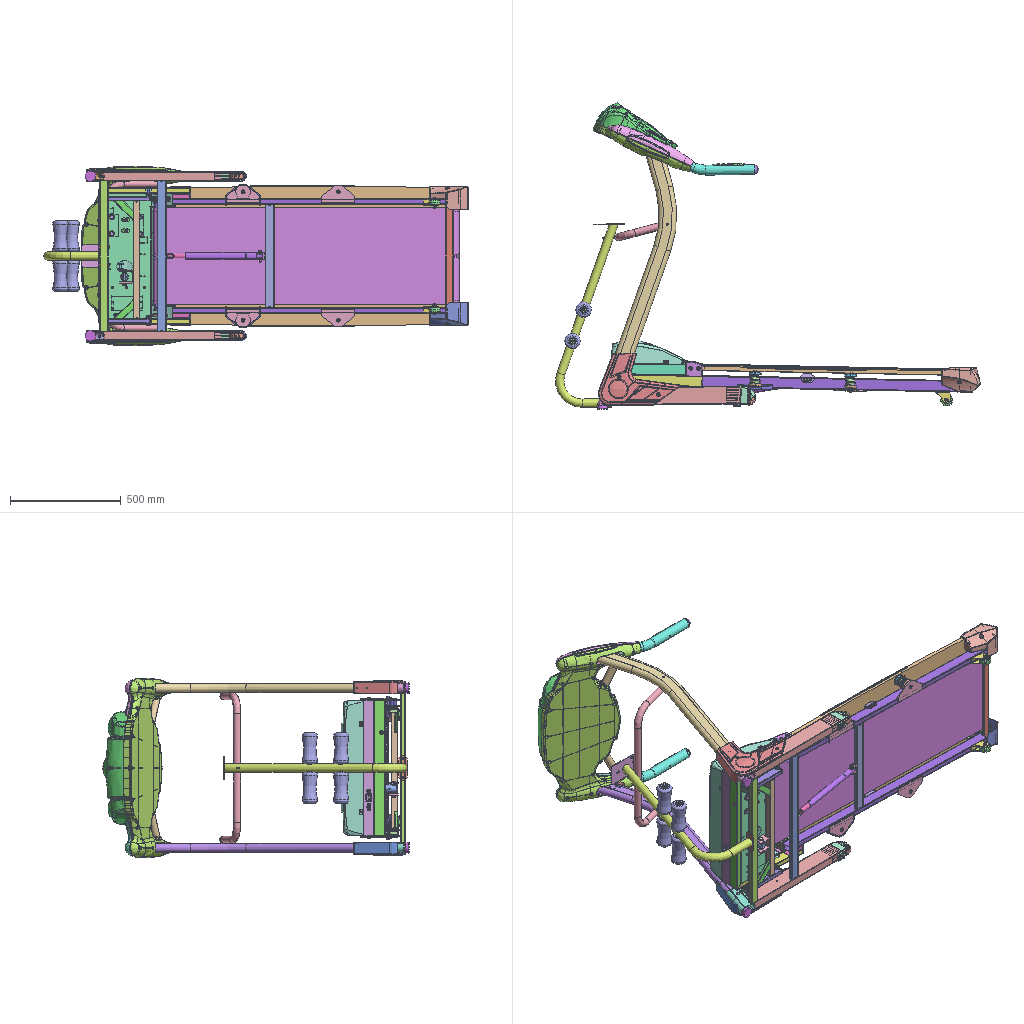Assembly | STEP file | 145 different items | 312 placed | box 1916 x 1381 x 810 mm
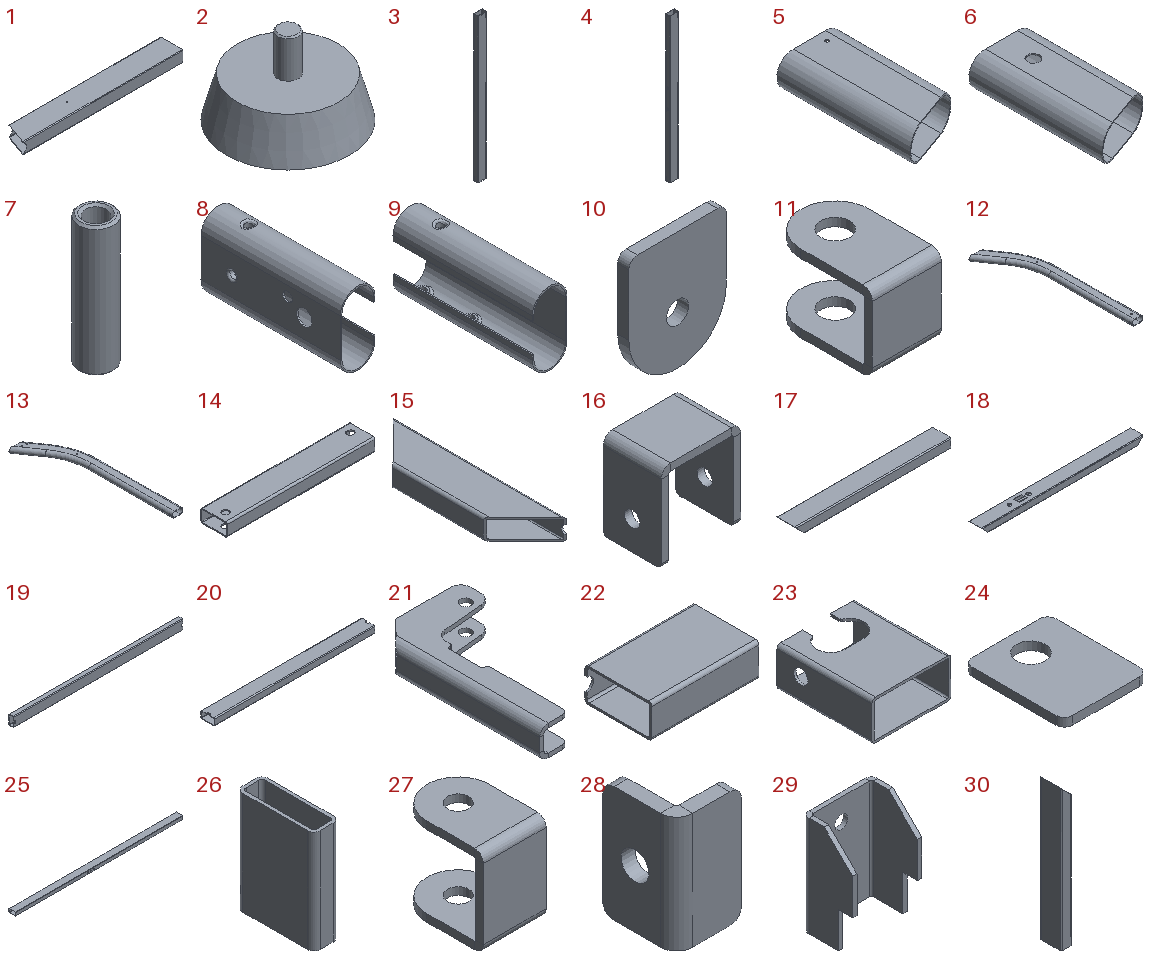Parts list (item | name | quantity | parent item | size | volume):
1 | 6150101 | x2 | in 6150100 | 569.929 x 80 x 40 mm | 191514 mm3
2 | 6150101W | x2 | in 6150100Z | 48.593 x 48.593 x 32 mm | 27204 mm3
3 | 6150102 | x1 | in 6150100 | 40 x 20 x 680 mm | 113098 mm3
4 | 6150103 | x1 | in 6150100 | 40 x 20 x 680 mm | 112626 mm3
5 | 6150104L | x1 | in 6150100 | 80 x 165 x 40 mm | 45327 mm3
6 | 6150104R | x1 | in 6150100 | 80 x 165 x 40 mm | 45081 mm3
7 | 6150104W | x2 | in 6150102LWZ, 6150102RWZ | 8.2 x 8.2 x 31 mm | 968.239 mm3
8 | 6150105L | x1 | in 6150100 | 36 x 145 x 76 mm | 34893 mm3
9 | 6150105R | x1 | in 6150100 | 36 x 145 x 76 mm | 34904 mm3
10 | 6150107 | x2 | in 6150100 | 35 x 4 x 42.5 mm | 5208 mm3
11 | 6150108 | x4 | in 6150100, 6150500 | 25 x 38.5 x 28 mm | 6374 mm3
12 | 6150201L | x1 | in 615 | 263.127 x 990.805 x 40 mm | 310034 mm3
13 | 6150201R | x1 | in 615 | 263.127 x 990.805 x 40 mm | 310034 mm3
14 | 6150402 | x2 | in 6150400 | 225 x 40 x 20 mm | 36971 mm3
15 | 6150403 | x2 | in 6150400 | 30 x 125 x 15 mm | 9413 mm3
16 | 6150404 | x1 | in 6150400 | 55 x 40 x 60 mm | 31409 mm3
17 | 6150501 | x2 | in 6150500 | 410 x 50 x 25 mm | 84495 mm3
18 | 6150502 | x1 | in 6150500 | 613 x 50 x 25 mm | 116984 mm3
19 | 6150504 | x1 | in 6150500 | 515 x 15 x 30 mm | 62451 mm3
20 | 6150505 | x1 | in 6150500 | 465 x 40 x 20 mm | 77302 mm3
21 | 6150506 | x1 | in 6150500 | 84 x 160 x 29 mm | 53248 mm3
22 | 6150507 | x2 | in 6150500 | 80 x 50 x 25 mm | 16946 mm3
23 | 6150508 | x1 | in 6150500 | 50 x 60 x 25 mm | 11554 mm3
24 | 6150509 | x1 | in 6150500 | 50 x 60 x 5 mm | 13731 mm3
25 | 6150510 | x2 | in 6150500 | 1235 x 50 x 25 mm | 262357 mm3
26 | 6150511 | x2 | in 6150500 | 10 x 30 x 40 mm | 3453 mm3
27 | 6150512 | x1 | in 6150500 | 25 x 35 x 35 mm | 6553 mm3
28 | 6150513 | x4 | in 6150500 | 14 x 16 x 25 mm | 1860 mm3
29 | 6150514 | x4 | in 6150500 | 48 x 35 x 70 mm | 19897 mm3
30 | 6150515 | x1 | in 6150500 | 25 x 50 x 334 mm | 67995 mm3
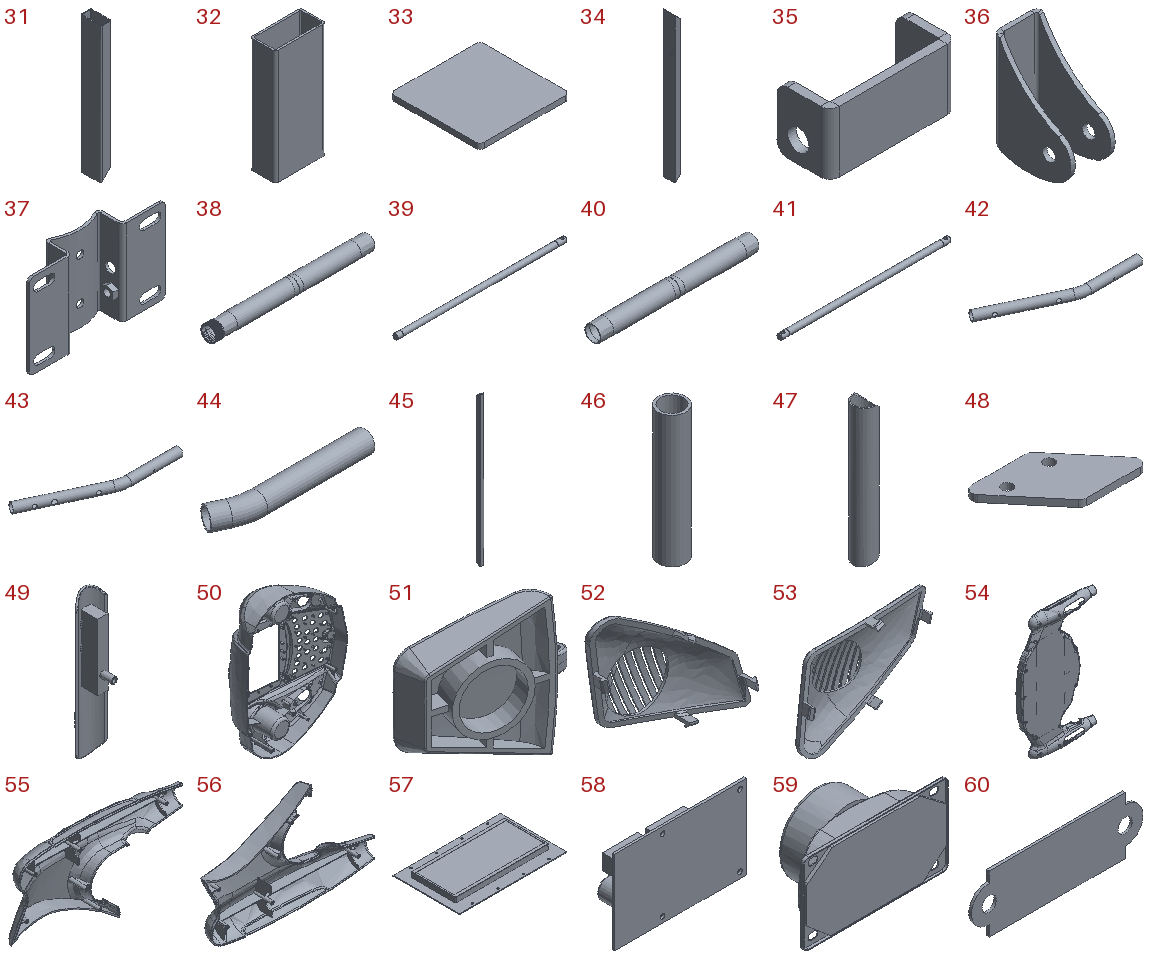31 | 6150516 | x1 | in 6150500 | 25 x 50 x 334 mm | 67613 mm3
32 | 6150517 | x2 | in 6150500 | 40 x 20 x 90 mm | 14984 mm3
33 | 6150518 | x2 | in 6150500 | 50 x 50 x 3 mm | 7484 mm3
34 | 6150519 | x1 | in 6150500 | 25 x 50 x 613 mm | 123960 mm3
35 | 6150521 | x2 | in 6150500 | 60 x 25 x 29 mm | 10869 mm3
36 | 6150522 | x2 | in 6150500 | 30 x 53 x 70.522 mm | 17329 mm3
37 | 6150601 | x1 | in 6150600Z | 160 x 30 x 100 mm | 59957 mm3
38 | 6150701 | x1 | in 6150700Z | 515 x 50 x 50 mm | 250147 mm3
39 | 6150702 | x1 | in 6150700Z | 565 x 17 x 17 mm | 128550 mm3
40 | 6150801 | x1 | in 6150800Z | 475 x 50 x 50 mm | 235448 mm3
41 | 6150802 | x1 | in 6150800Z | 523 x 17 x 17 mm | 116773 mm3
42 | 6151201L | x1 | in 6151200 | 584.322 x 188.458 x 38.1 mm | 101738 mm3
43 | 6151201R | x1 | in 6151200 | 584.322 x 188.458 x 38.1 mm | 101253 mm3
44 | 6151201WA | x2 | in 6151200Z | 313.697 x 67.391 x 44.1 mm | 119753 mm3
45 | 6151202 | x1 | in 6151200 | 20 x 20 x 700 mm | 73457 mm3
46 | 6151202W | x2 | in 6151200Z | 34.6 x 34.6 x 165 mm | 49141 mm3
47 | 6151203 | x2 | in 6151200 | 28.6 x 28.6 x 183 mm | 22465 mm3
48 | 6151204 | x2 | in 6151200 | 82.726 x 50 x 5 mm | 12291 mm3
49 | 6151204W | x2 | in 6151200Z | 31 x 32.516 x 144.3 mm | 20924 mm3
50 | 6151206W | x1 | in 6151200A | 380 x 123.405 x 510 mm | 795942 mm3
51 | 6151207W | x1 | in 6151200A | 35.148 x 15.37 x 38.312 mm | 3411 mm3
52 | 6151208LW | x1 | in 6151200A | 94.278 x 29.99 x 86.4 mm | 11134 mm3
53 | 6151208RW | x1 | in 6151200A | 94.278 x 29.99 x 86.4 mm | 11135 mm3
54 | 6151209W | x1 | in 6151200A | - | -
55 | 6151210LW | x1 | in 6151200A | 418.826 x 58.845 x 246.762 mm | 255227 mm3
56 | 6151210RW | x1 | in 6151200A | 418.823 x 58.845 x 246.762 mm | 256127 mm3
57 | 6151211W | x1 | in 6151200A | 210 x 130 x 11.5 mm | 192424 mm3
58 | 6151212W | x1 | in 6151200A | 85 x 25.5 x 54 mm | 22602 mm3
59 | 6151213W | x2 | in 6151200A | 90 x 37.5 x 50 mm | 46130 mm3
60 | 6151214W | x1 | in 6151200A | 48 x 0.7 x 16 mm | 462.985 mm3
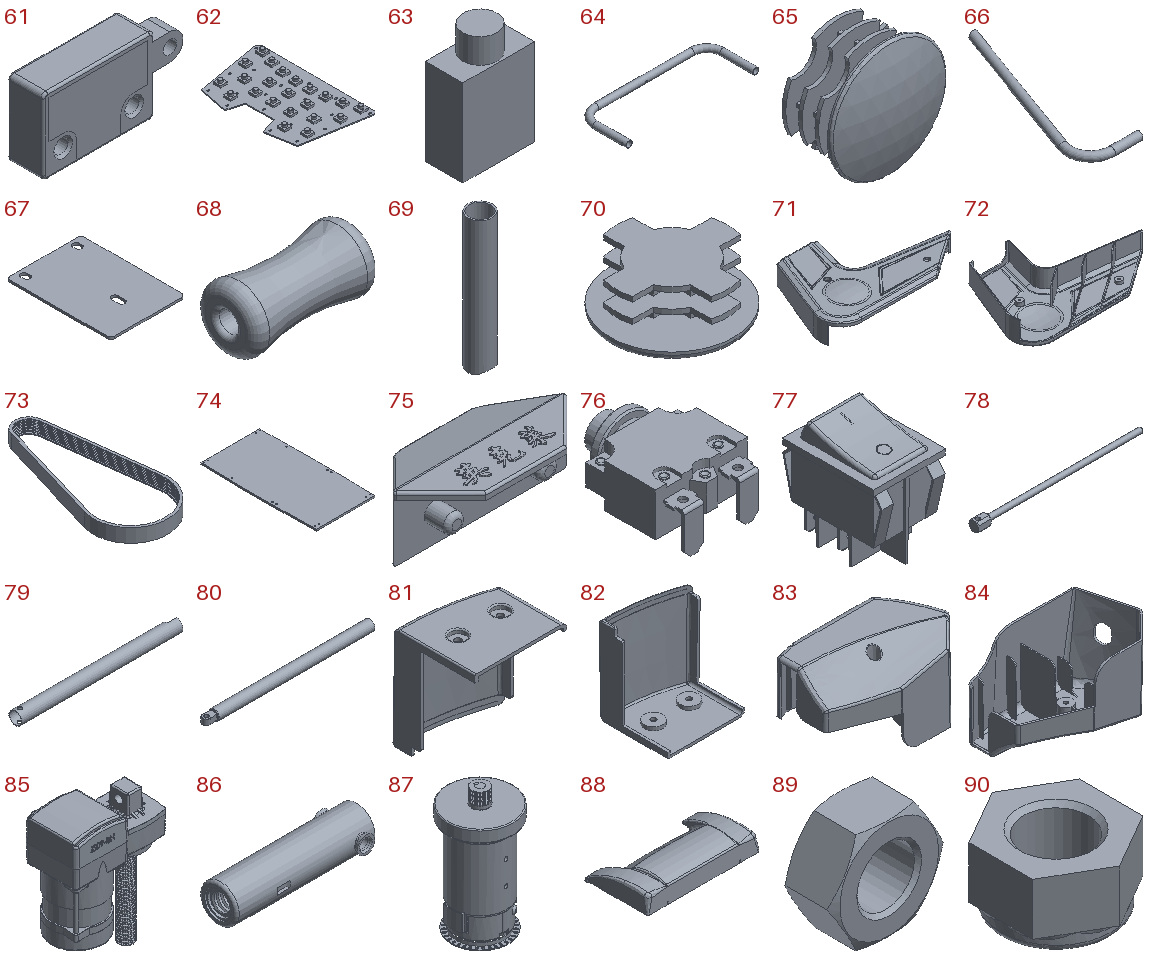61 | 6151215W | x1 | in 6151200A | 31.5 x 8 x 17 mm | 3233 mm3
62 | 6151216W | x1 | in 6151200A | 123.89 x 199.336 x 9.1 mm | 46747 mm3
63 | 6151217W | x1 | in 6151200A | 11.5 x 6 x 18 mm | 1061 mm3
64 | 6151301 | x1 | in 6151300 | 679.8 x 265.9 x 31.8 mm | 153699 mm3
65 | 6151301W | x2 | in 6151300Z | 31.8 x 17.071 x 31.8 mm | 4059 mm3
66 | 6151401 | x1 | in 6151400 | 289.236 x 823.315 x 38.1 mm | 178322 mm3
67 | 6151403 | x1 | in 6151400 | 100 x 140 x 3 mm | 40958 mm3
68 | 6151403W | x4 | in 6151400Z | 140 x 70 x 70 mm | 348651 mm3
69 | 6151404 | x4 | in 6151400 | 25.4 x 25.4 x 140 mm | 15577 mm3
70 | 6151404W | x4 | in 6151400Z | 25.4 x 25.4 x 10 mm | 1636 mm3
71 | BLZHT2-L | x1 | in 615 | 369.553 x 235 x 62.57 mm | 247384 mm3
72 | BLZHT2-R | x1 | in 615 | 369.553 x 235 x 62.57 mm | 247382 mm3
73 | DE200J618 | x1 | in 6150500Z | 99 x 216 x 18 mm | 21820 mm3
74 | DECAK 615 | x1 | in 6150500Z | 633 x 1220 x 18 mm | 13739057 mm3
75 | DECH07 | x2 | in 6150500Z | 74.172 x 40 x 28.5 mm | 30644 mm3
76 | EC002 | x1 | in 6150500Z | 29.3 x 39.3 x 19.65 mm | 10331 mm3
77 | EP002 | x1 | in 6150500Z | 25 x 34.5 x 34.784 mm | 14567 mm3
78 | GAS SHOCK 608S | x1 | in 615 | 353.5 x 20 x 20 mm | 34694 mm3
79 | GAS SHOCK 608W | x1 | in 615 | 353 x 28 x 28 mm | 42661 mm3
80 | GAS SHOCK 608X | x1 | in 615 | 359 x 22 x 22 mm | 94119 mm3
81 | HGL | x1 | in 6150500Z | 76.869 x 67.947 x 85 mm | 33917 mm3
82 | HGR | x1 | in 6150500Z | 76.869 x 67.947 x 85 mm | 33917 mm3
83 | HHJL | x1 | in 6150500Z | 176.285 x 110 x 105 mm | 139375 mm3
84 | HHJR | x1 | in 6150500Z | 176.285 x 110 x 105.001 mm | 141241 mm3
85 | JS09-BN 618 | x1 | in 615 | 127.975 x 72.828 x 177.5 mm | 665707 mm3
86 | JS09-BNB 618 | x1 | in 615 | 130.5 x 41.999 x 35 mm | 51748 mm3
87 | MOTOR 618 | x1 | in 6150600Z | - | -
88 | MOTOR COVER | x1 | in 6150500Z | 627.004 x 340 x 102.717 mm | 823151 mm3
89 | N108078 | x8 | in 6150100, 6150500, 6151300 | 16.166 x 7 x 14 mm | 821.972 mm3
90 | N210095 | x10 | in 615, 6150500Z | 17 x 19.63 x 10.5 mm | 1722 mm3
91 | PL6203ZZA_default | x4 | in 6150700Z, 6150800Z | - | -
92 | PN_0001 | x4 | in 6150500Z | - | -
93 | PN_0002 | x2 | in 6150102LWZ, 6150102RWZ | - | -
94 | PN_0003 | x4 | in 6150700Z, 6150800Z | - | -
95 | PN_0004 | x2 | in 6150102LWZ, 6150102RWZ | - | -
96 | PN_0005_default | x4 | in 6150500Z | - | -
97 | PN_0006_default | x1 | in 6150700Z | - | -
98 | PN_0007_default | x4 | in 6150500Z | - | -
99 | PN_0008_default | x4 | in 6150500 | - | -
100 | PN_0009 | x4 | in 615 | - | -
101 | PN_0010 | x4 | in 6150500Z | - | -
102 | PN_0011_default | x4 | in 615 | - | -
103 | PN_0012 | x7 | in 615, 6150500Z | - | -
104 | PN_0013_default | x4 | in 6150500Z | - | -
105 | PN_0014 | x13 | in 615, 6150500Z | - | -
106 | PN_0015 | x8 | in 6150500Z | - | -
107 | PN_0016 | x2 | in 6150500Z | - | -
108 | PN_0017_default | x1 | in 6150500Z | - | -
109 | PN_0018_default | x1 | in 6151400 | - | -
110 | PN_0019 | x4 | in 6150500Z | - | -
111 | PN_0020 | x7 | in 615, 6150500Z | - | -
112 | PN_0021_default | x2 | in 6150102LWZ, 6150102RWZ | - | -
113 | PN_0022 | x2 | in 6150500Z | - | -
114 | PN_0023 | x1 | in 6150500Z | - | -
115 | PN_0024_default | x1 | in 6150400 | - | -
116 | PN_0025_default | x1 | in 6150500Z | - | -
117 | PN_0026_default | x1 | in 6150100 | - | -
118 | PN_0027_default | x2 | in 6150102LWZ, 6150102RWZ | - | -
119 | PN_0028_default | x1 | in 6150500 | - | -
120 | PN_0029_default | x1 | in 6150500Z | - | -
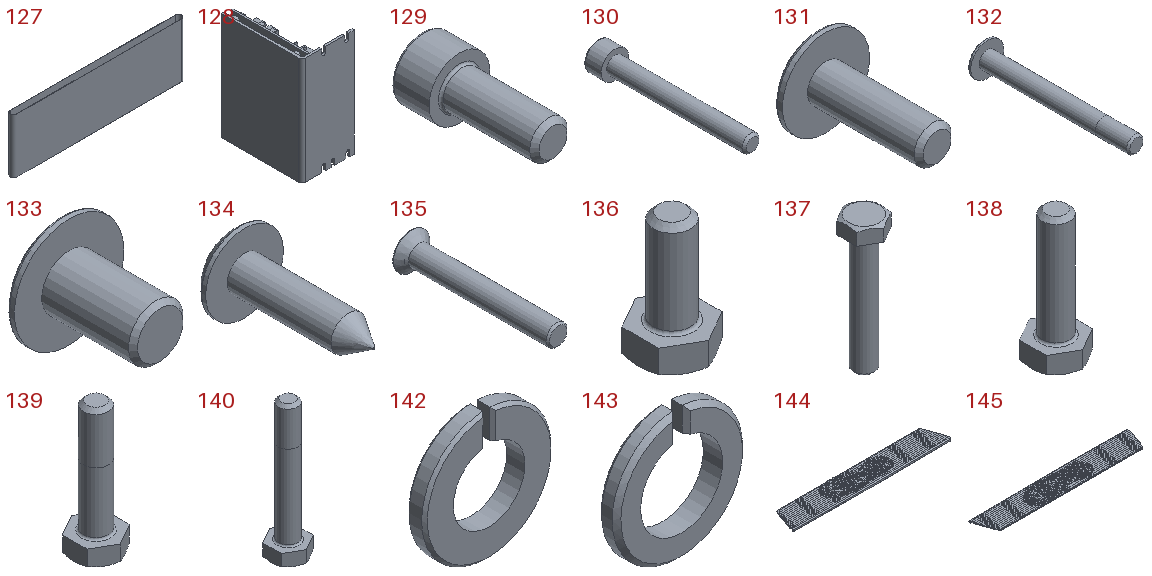121 | PN_0030_default | x2 | in 6150500Z | - | -
122 | PN_0031_default | x2 | in 6151200Z | - | -
123 | PN_0032_default | x4 | in 6150500Z | - | -
124 | PN_0033 | x5 | in 6150500Z | - | -
125 | PN_0034 | x1 | in 615 | - | -
126 | Polyester film | x1 | in 6150500Z | - | -
127 | RUBE 615 | x1 | in 6150500Z | 1381 x 53.2 x 440 mm | 1983947 mm3
128 | RUNMCI-615 | x1 | in 6150500Z | 68 x 105 x 140 mm | 172044 mm3
129 | SA10820 | x2 | in 6150600Z | 13 x 28 x 13 mm | 1908 mm3
130 | SA10865 | x3 | in 6150500Z | 13 x 73 x 13 mm | 4160 mm3
131 | SD10412 | x5 | in 6150500Z | 9.4 x 14.503 x 9.4 mm | 245.335 mm3
132 | SD10545 | x2 | in 6150102LWZ, 6150102RWZ | 10 x 47.433 x 10 mm | 991.806 mm3
133 | SD10610 | x3 | in 6150500Z | 12 x 12.964 x 12 mm | 479.053 mm3
134 | SD20415 | x1 | in 6150500Z | 9 x 17.646 x 9 mm | 255.973 mm3
135 | SD30640 | x4 | in 6150500Z | 10.421 x 42.38 x 10.421 mm | 1245 mm3
136 | SI1025_M10 | x4 | in 6150500Z | 17 x 19.6 x 32 mm | 3678 mm3
137 | SI10845 | x1 | in 615 | 13 x 15.011 x 50.5 mm | 3048 mm3
138 | SI11035_M10 | x4 | in 615 | 17 x 19.6 x 47 mm | 4857 mm3
139 | SI11045_M10 | x1 | in 615 | 17 x 19.6 x 52 mm | 5249 mm3
140 | SI11065_M10 | x1 | in 615 | 17 x 19.6 x 72 mm | 6820 mm3
141 | Shock-absorbing sponge | x1 | in 6150500Z | - | -
142 | W204009 | x5 | in 6150500Z | 9.2 x 1.3 x 9.193 mm | 57.255 mm3
143 | W208016 | x10 | in 6150500Z, 6150600Z | 13.5 x 2 x 13.481 mm | 158.687 mm3
144 | ZHD 500.80L | x1 | in 6150500Z | 540 x 85 x 12 mm | 102957 mm3
145 | ZHD 500.80R | x1 | in 6150500Z | 540 x 85 x 12 mm | 102957 mm3